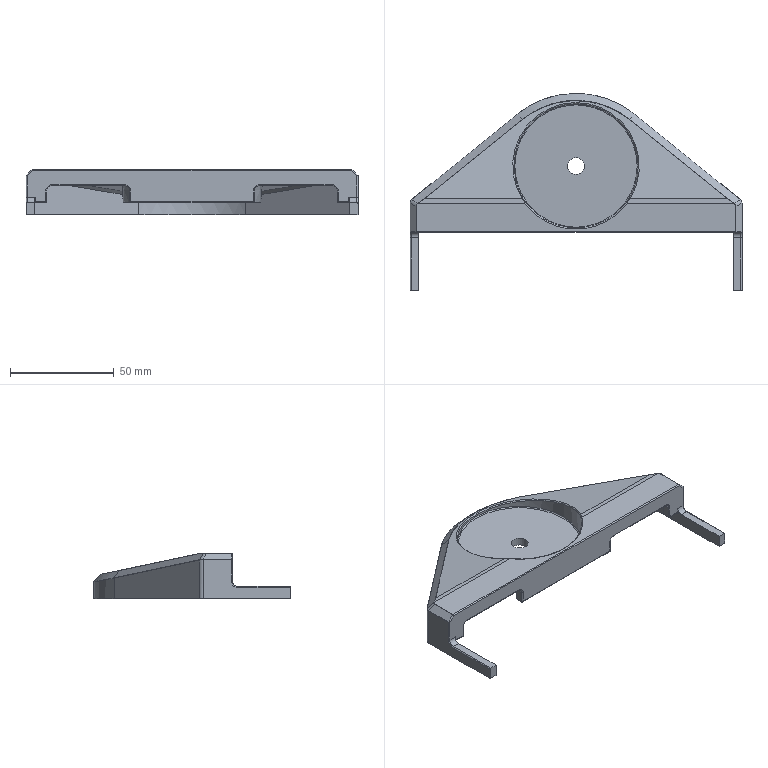Part | STEP file | PN_0013_default | 1 solid | 130 faces | box 160 x 95 x 22 mm | volume 49068 mm3 | cylinder 50 | plane 40 | spline 26 | torus 12 | cone 2 | commonest cylinder face diameters 1 x22 0.4 x10 5 x10 12 x2 20 x2 8.2 x1